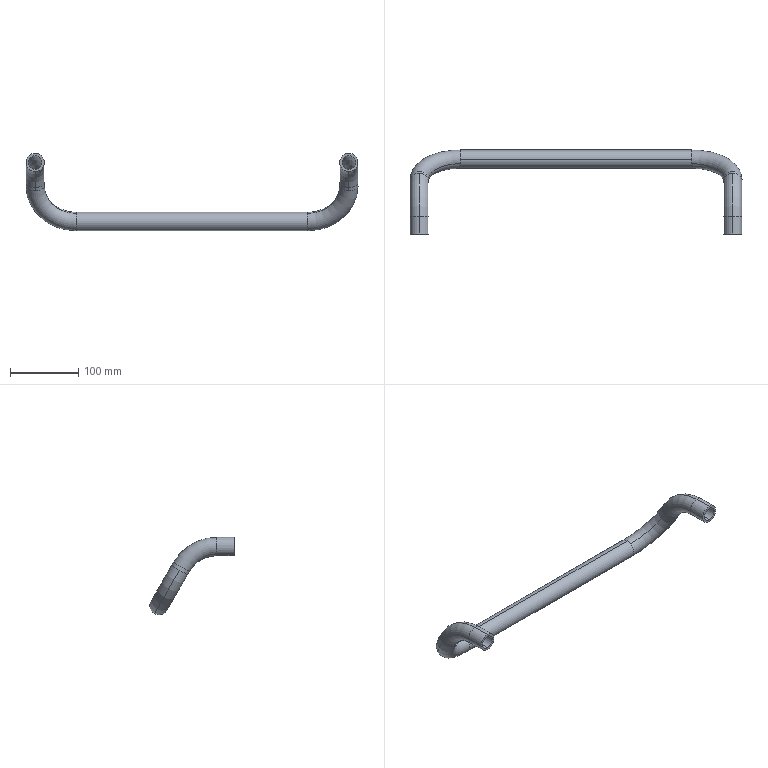Part | STEP file | X77-09101 | 1 solid | 38 faces | box 487 x 123.546 x 113.683 mm | volume 184955 mm3 | cylinder 20 | torus 16 | plane 2 | commonest cylinder face diameters 20 x10 27 x10
STEP:
#1=CARTESIAN_POINT('',(460.,25.359,10.));
#2=VERTEX_POINT('',#1);
#3=CARTESIAN_POINT('',(460.,25.359,-10.));
#4=VERTEX_POINT('',#3);
#5=CARTESIAN_POINT('',(460.,25.359,0.));
#6=DIRECTION('',(0.,1.,0.));
#7=DIRECTION('',(0.,0.,1.));
#8=AXIS2_PLACEMENT_3D('',#5,#6,#7);
#9=CIRCLE('',#8,10.);
#10=EDGE_CURVE('',#2,#4,#9,.T.);
#11=ORIENTED_EDGE('',*,*,#10,.F.);
#12=CARTESIAN_POINT('',(460.,85.981,-25.));
#13=VERTEX_POINT('',#12);
#14=CARTESIAN_POINT('',(460.,25.359,-60.));
#15=DIRECTION('',(-1.,0.,0.));
#16=DIRECTION('',(0.,0.,1.));
#17=AXIS2_PLACEMENT_3D('',#14,#15,#16);
#18=CIRCLE('',#17,70.);
#19=EDGE_CURVE('',#2,#13,#18,.T.);
#20=ORIENTED_EDGE('',*,*,#19,.T.);
#21=CARTESIAN_POINT('',(460.,68.66,-35.));
#22=VERTEX_POINT('',#21);
#23=CARTESIAN_POINT('',(460.,77.321,-30.));
#24=DIRECTION('',(0.,0.5,-0.866));
#25=DIRECTION('',(0.,0.866,0.5));
#26=AXIS2_PLACEMENT_3D('',#23,#24,#25);
#27=CIRCLE('',#26,10.);
#28=EDGE_CURVE('',#13,#22,#27,.T.);
#29=ORIENTED_EDGE('',*,*,#28,.T.);
#30=CARTESIAN_POINT('',(460.,25.359,-60.));
#31=DIRECTION('',(-1.,0.,0.));
#32=DIRECTION('',(0.,0.,1.));
#33=AXIS2_PLACEMENT_3D('',#30,#31,#32);
#34=CIRCLE('',#33,50.);
#35=EDGE_CURVE('',#4,#22,#34,.T.);
#36=ORIENTED_EDGE('',*,*,#35,.F.);
#37=EDGE_LOOP('',(#11,#20,#29,#36));
#38=FACE_OUTER_BOUND('',#37,.T.);
#39=CARTESIAN_POINT('',(460.,25.359,-60.));
#40=DIRECTION('',(-1.,0.,0.));
#41=DIRECTION('',(0.,0.,1.));
#42=AXIS2_PLACEMENT_3D('',#39,#40,#41);
#43=TOROIDAL_SURFACE('',#42,60.,10.);
#44=ADVANCED_FACE('',(#38),#43,.F.);
#45=CARTESIAN_POINT('',(460.,25.359,-13.5));
#46=VERTEX_POINT('',#45);
#47=CARTESIAN_POINT('',(460.,25.359,13.5));
#48=VERTEX_POINT('',#47);
#49=CARTESIAN_POINT('',(460.,25.359,0.));
#50=DIRECTION('',(0.,1.,0.));
#51=DIRECTION('',(0.,0.,1.));
#52=AXIS2_PLACEMENT_3D('',#49,#50,#51);
#53=CIRCLE('',#52,13.5);
#54=EDGE_CURVE('',#46,#48,#53,.T.);
#55=ORIENTED_EDGE('',*,*,#54,.T.);
#56=CARTESIAN_POINT('',(460.,89.012,-23.25));
#57=VERTEX_POINT('',#56);
#58=CARTESIAN_POINT('',(460.,25.359,-60.));
#59=DIRECTION('',(-1.,0.,0.));
#60=DIRECTION('',(0.,0.,1.));
#61=AXIS2_PLACEMENT_3D('',#58,#59,#60);
#62=CIRCLE('',#61,73.5);
#63=EDGE_CURVE('',#48,#57,#62,.T.);
#64=ORIENTED_EDGE('',*,*,#63,.T.);
#65=CARTESIAN_POINT('',(460.,65.629,-36.75));
#66=VERTEX_POINT('',#65);
#67=CARTESIAN_POINT('',(460.,77.321,-30.));
#68=DIRECTION('',(0.,0.5,-0.866));
#69=DIRECTION('',(0.,0.866,0.5));
#70=AXIS2_PLACEMENT_3D('',#67,#68,#69);
#71=CIRCLE('',#70,13.5);
#72=EDGE_CURVE('',#66,#57,#71,.T.);
#73=ORIENTED_EDGE('',*,*,#72,.F.);
#74=CARTESIAN_POINT('',(460.,25.359,-60.));
#75=DIRECTION('',(-1.,0.,0.));
#76=DIRECTION('',(0.,0.,1.));
#77=AXIS2_PLACEMENT_3D('',#74,#75,#76);
#78=CIRCLE('',#77,46.5);
#79=EDGE_CURVE('',#46,#66,#78,.T.);
#80=ORIENTED_EDGE('',*,*,#79,.F.);
#81=EDGE_LOOP('',(#55,#64,#73,#80));
#82=FACE_OUTER_BOUND('',#81,.T.);
#83=CARTESIAN_POINT('',(460.,25.359,-60.));
#84=DIRECTION('',(-1.,0.,0.));
#85=DIRECTION('',(0.,0.,1.));
#86=AXIS2_PLACEMENT_3D('',#83,#84,#85);
#87=TOROIDAL_SURFACE('',#86,60.,13.5);
#88=ADVANCED_FACE('',(#82),#87,.T.);
#89=CARTESIAN_POINT('',(470.,80.046,-34.721));
#90=VERTEX_POINT('',#89);
#91=CARTESIAN_POINT('',(460.,71.386,-39.721));
#92=VERTEX_POINT('',#91);
#93=CARTESIAN_POINT('',(460.,80.046,-34.721));
#94=DIRECTION('',(0.,0.5,-0.866));
#95=DIRECTION('',(0.,0.866,0.5));
#96=AXIS2_PLACEMENT_3D('',#93,#94,#95);
#97=CIRCLE('',#96,10.);
#98=EDGE_CURVE('',#90,#92,#97,.T.);
#99=ORIENTED_EDGE('',*,*,#98,.F.);
#100=CARTESIAN_POINT('',(400.,115.046,-95.343));
#101=VERTEX_POINT('',#100);
#102=CARTESIAN_POINT('',(400.,80.046,-34.721));
#103=DIRECTION('',(0.,0.866,0.5));
#104=DIRECTION('',(0.,-0.5,0.866));
#105=AXIS2_PLACEMENT_3D('',#102,#103,#104);
#106=CIRCLE('',#105,70.);
#107=EDGE_CURVE('',#90,#101,#106,.T.);
#108=ORIENTED_EDGE('',*,*,#107,.T.);
#109=CARTESIAN_POINT('',(400.,110.046,-96.683));
#110=VERTEX_POINT('',#109);
#111=CARTESIAN_POINT('',(400.,110.046,-86.683));
#112=DIRECTION('',(-1.,0.,0.));
#113=DIRECTION('',(0.,0.866,0.5));
#114=AXIS2_PLACEMENT_3D('',#111,#112,#113);
#115=CIRCLE('',#114,10.);
#116=EDGE_CURVE('',#101,#110,#115,.T.);
#117=ORIENTED_EDGE('',*,*,#116,.T.);
#118=CARTESIAN_POINT('',(400.,105.046,-78.023));
#119=VERTEX_POINT('',#118);
#120=CARTESIAN_POINT('',(400.,110.046,-86.683));
#121=DIRECTION('',(-1.,0.,0.));
#122=DIRECTION('',(0.,0.866,0.5));
#123=AXIS2_PLACEMENT_3D('',#120,#121,#122);
#124=CIRCLE('',#123,10.);
#125=EDGE_CURVE('',#110,#119,#124,.T.);
#126=ORIENTED_EDGE('',*,*,#125,.T.);
#127=CARTESIAN_POINT('',(450.,80.046,-34.721));
#128=VERTEX_POINT('',#127);
#129=CARTESIAN_POINT('',(400.,80.046,-34.721));
#130=DIRECTION('',(0.,0.866,0.5));
#131=DIRECTION('',(0.,-0.5,0.866));
#132=AXIS2_PLACEMENT_3D('',#129,#130,#131);
#133=CIRCLE('',#132,50.);
#134=EDGE_CURVE('',#128,#119,#133,.T.);
#135=ORIENTED_EDGE('',*,*,#134,.F.);
#136=CARTESIAN_POINT('',(460.,80.046,-34.721));
#137=DIRECTION('',(0.,0.5,-0.866));
#138=DIRECTION('',(0.,0.866,0.5));
#139=AXIS2_PLACEMENT_3D('',#136,#137,#138);
#140=CIRCLE('',#139,10.);
#141=EDGE_CURVE('',#92,#128,#140,.T.);
#142=ORIENTED_EDGE('',*,*,#141,.F.);
#143=EDGE_LOOP('',(#99,#108,#117,#126,#135,#142));
#144=FACE_OUTER_BOUND('',#143,.T.);
#145=CARTESIAN_POINT('',(400.,80.046,-34.721));
#146=DIRECTION('',(0.,0.866,0.5));
#147=DIRECTION('',(0.,-0.5,0.866));
#148=AXIS2_PLACEMENT_3D('',#145,#146,#147);
#149=TOROIDAL_SURFACE('',#148,60.,10.);
#150=ADVANCED_FACE('',(#144),#149,.F.);
#151=CARTESIAN_POINT('',(460.,91.738,-27.971));
#152=VERTEX_POINT('',#151);
#153=CARTESIAN_POINT('',(473.5,80.046,-34.721));
#154=VERTEX_POINT('',#153);
#155=CARTESIAN_POINT('',(460.,80.046,-34.721));
#156=DIRECTION('',(0.,0.5,-0.866));
#157=DIRECTION('',(0.,0.866,0.5));
#158=AXIS2_PLACEMENT_3D('',#155,#156,#157);
#159=CIRCLE('',#158,13.5);
#160=EDGE_CURVE('',#152,#154,#159,.T.);
#161=ORIENTED_EDGE('',*,*,#160,.T.);
#162=CARTESIAN_POINT('',(400.,116.796,-98.374));
#163=VERTEX_POINT('',#162);
#164=CARTESIAN_POINT('',(400.,80.046,-34.721));
#165=DIRECTION('',(0.,0.866,0.5));
#166=DIRECTION('',(0.,-0.5,0.866));
#167=AXIS2_PLACEMENT_3D('',#164,#165,#166);
#168=CIRCLE('',#167,73.5);
#169=EDGE_CURVE('',#154,#163,#168,.T.);
#170=ORIENTED_EDGE('',*,*,#169,.T.);
#171=CARTESIAN_POINT('',(400.,110.046,-73.183));
#172=VERTEX_POINT('',#171);
#173=CARTESIAN_POINT('',(400.,110.046,-86.683));
#174=DIRECTION('',(-1.,0.,0.));
#175=DIRECTION('',(0.,0.866,0.5));
#176=AXIS2_PLACEMENT_3D('',#173,#174,#175);
#177=CIRCLE('',#176,13.5);
#178=EDGE_CURVE('',#172,#163,#177,.T.);
#179=ORIENTED_EDGE('',*,*,#178,.F.);
#180=CARTESIAN_POINT('',(400.,103.296,-74.992));
#181=VERTEX_POINT('',#180);
#182=CARTESIAN_POINT('',(400.,110.046,-86.683));
#183=DIRECTION('',(-1.,0.,0.));
#184=DIRECTION('',(0.,0.866,0.5));
#185=AXIS2_PLACEMENT_3D('',#182,#183,#184);
#186=CIRCLE('',#185,13.5);
#187=EDGE_CURVE('',#181,#172,#186,.T.);
#188=ORIENTED_EDGE('',*,*,#187,.F.);
#189=CARTESIAN_POINT('',(446.5,80.046,-34.721));
#190=VERTEX_POINT('',#189);
#191=CARTESIAN_POINT('',(400.,80.046,-34.721));
#192=DIRECTION('',(0.,0.866,0.5));
#193=DIRECTION('',(0.,-0.5,0.866));
#194=AXIS2_PLACEMENT_3D('',#191,#192,#193);
#195=CIRCLE('',#194,46.5);
#196=EDGE_CURVE('',#190,#181,#195,.T.);
#197=ORIENTED_EDGE('',*,*,#196,.F.);
#198=CARTESIAN_POINT('',(460.,80.046,-34.721));
#199=DIRECTION('',(0.,0.5,-0.866));
#200=DIRECTION('',(0.,0.866,0.5));
#201=AXIS2_PLACEMENT_3D('',#198,#199,#200);
#202=CIRCLE('',#201,13.5);
#203=EDGE_CURVE('',#190,#152,#202,.T.);
#204=ORIENTED_EDGE('',*,*,#203,.T.);
#205=EDGE_LOOP('',(#161,#170,#179,#188,#197,#204));
#206=FACE_OUTER_BOUND('',#205,.T.);
#207=CARTESIAN_POINT('',(400.,80.046,-34.721));
#208=DIRECTION('',(0.,0.866,0.5));
#209=DIRECTION('',(0.,-0.5,0.866));
#210=AXIS2_PLACEMENT_3D('',#207,#208,#209);
#211=TOROIDAL_SURFACE('',#210,60.,13.5);
#212=ADVANCED_FACE('',(#206),#211,.T.);
#213=CARTESIAN_POINT('',(60.,115.046,-95.343));
#214=VERTEX_POINT('',#213);
#215=CARTESIAN_POINT('',(60.,110.046,-96.683));
#216=VERTEX_POINT('',#215);
#217=CARTESIAN_POINT('',(60.,110.046,-86.683));
#218=DIRECTION('',(-1.,0.,0.));
#219=DIRECTION('',(0.,0.866,0.5));
#220=AXIS2_PLACEMENT_3D('',#217,#218,#219);
#221=CIRCLE('',#220,10.);
#222=EDGE_CURVE('',#214,#216,#221,.T.);
#223=ORIENTED_EDGE('',*,*,#222,.F.);
#224=CARTESIAN_POINT('',(-10.,80.046,-34.721));
#225=VERTEX_POINT('',#224);
#226=CARTESIAN_POINT('',(60.,80.046,-34.721));
#227=DIRECTION('',(0.,0.866,0.5));
#228=DIRECTION('',(0.,-0.5,0.866));
#229=AXIS2_PLACEMENT_3D('',#226,#227,#228);
#230=CIRCLE('',#229,70.);
#231=EDGE_CURVE('',#214,#225,#230,.T.);
#232=ORIENTED_EDGE('',*,*,#231,.T.);
#233=CARTESIAN_POINT('',(0.,71.386,-39.721));
#234=VERTEX_POINT('',#233);
#235=CARTESIAN_POINT('',(0.,80.046,-34.721));
#236=DIRECTION('',(0.,-0.5,0.866));
#237=DIRECTION('',(0.,0.866,0.5));
#238=AXIS2_PLACEMENT_3D('',#235,#236,#237);
#239=CIRCLE('',#238,10.);
#240=EDGE_CURVE('',#225,#234,#239,.T.);
#241=ORIENTED_EDGE('',*,*,#240,.T.);
#242=CARTESIAN_POINT('',(10.,80.046,-34.721));
#243=VERTEX_POINT('',#242);
#244=CARTESIAN_POINT('',(0.,80.046,-34.721));
#245=DIRECTION('',(0.,-0.5,0.866));
#246=DIRECTION('',(0.,0.866,0.5));
#247=AXIS2_PLACEMENT_3D('',#244,#245,#246);
#248=CIRCLE('',#247,10.);
#249=EDGE_CURVE('',#234,#243,#248,.T.);
#250=ORIENTED_EDGE('',*,*,#249,.T.);
#251=CARTESIAN_POINT('',(60.,105.046,-78.023));
#252=VERTEX_POINT('',#251);
#253=CARTESIAN_POINT('',(60.,80.046,-34.721));
#254=DIRECTION('',(0.,0.866,0.5));
#255=DIRECTION('',(0.,-0.5,0.866));
#256=AXIS2_PLACEMENT_3D('',#253,#254,#255);
#257=CIRCLE('',#256,50.);
#258=EDGE_CURVE('',#252,#243,#257,.T.);
#259=ORIENTED_EDGE('',*,*,#258,.F.);
#260=CARTESIAN_POINT('',(60.,110.046,-86.683));
#261=DIRECTION('',(-1.,0.,0.));
#262=DIRECTION('',(0.,0.866,0.5));
#263=AXIS2_PLACEMENT_3D('',#260,#261,#262);
#264=CIRCLE('',#263,10.);
#265=EDGE_CURVE('',#216,#252,#264,.T.);
#266=ORIENTED_EDGE('',*,*,#265,.F.);
#267=EDGE_LOOP('',(#223,#232,#241,#250,#259,#266));
#268=FACE_OUTER_BOUND('',#267,.T.);
#269=CARTESIAN_POINT('',(60.,80.046,-34.721));
#270=DIRECTION('',(0.,0.866,0.5));
#271=DIRECTION('',(0.,-0.5,0.866));
#272=AXIS2_PLACEMENT_3D('',#269,#270,#271);
#273=TOROIDAL_SURFACE('',#272,60.,10.);
#274=ADVANCED_FACE('',(#268),#273,.F.);
#275=CARTESIAN_POINT('',(60.,110.046,-73.183));
#276=VERTEX_POINT('',#275);
#277=CARTESIAN_POINT('',(60.,116.796,-98.374));
#278=VERTEX_POINT('',#277);
#279=CARTESIAN_POINT('',(60.,110.046,-86.683));
#280=DIRECTION('',(-1.,0.,0.));
#281=DIRECTION('',(0.,0.866,0.5));
#282=AXIS2_PLACEMENT_3D('',#279,#280,#281);
#283=CIRCLE('',#282,13.5);
#284=EDGE_CURVE('',#276,#278,#283,.T.);
#285=ORIENTED_EDGE('',*,*,#284,.T.);
#286=CARTESIAN_POINT('',(-13.5,80.046,-34.721));
#287=VERTEX_POINT('',#286);
#288=CARTESIAN_POINT('',(60.,80.046,-34.721));
#289=DIRECTION('',(0.,0.866,0.5));
#290=DIRECTION('',(0.,-0.5,0.866));
#291=AXIS2_PLACEMENT_3D('',#288,#289,#290);
#292=CIRCLE('',#291,73.5);
#293=EDGE_CURVE('',#278,#287,#292,.T.);
#294=ORIENTED_EDGE('',*,*,#293,.T.);
#295=CARTESIAN_POINT('',(0.,91.738,-27.971));
#296=VERTEX_POINT('',#295);
#297=CARTESIAN_POINT('',(0.,80.046,-34.721));
#298=DIRECTION('',(0.,-0.5,0.866));
#299=DIRECTION('',(0.,0.866,0.5));
#300=AXIS2_PLACEMENT_3D('',#297,#298,#299);
#301=CIRCLE('',#300,13.5);
#302=EDGE_CURVE('',#296,#287,#301,.T.);
#303=ORIENTED_EDGE('',*,*,#302,.F.);
#304=CARTESIAN_POINT('',(13.5,80.046,-34.721));
#305=VERTEX_POINT('',#304);
#306=CARTESIAN_POINT('',(0.,80.046,-34.721));
#307=DIRECTION('',(0.,-0.5,0.866));
#308=DIRECTION('',(0.,0.866,0.5));
#309=AXIS2_PLACEMENT_3D('',#306,#307,#308);
#310=CIRCLE('',#309,13.5);
#311=EDGE_CURVE('',#305,#296,#310,.T.);
#312=ORIENTED_EDGE('',*,*,#311,.F.);
#313=CARTESIAN_POINT('',(60.,103.296,-74.992));
#314=VERTEX_POINT('',#313);
#315=CARTESIAN_POINT('',(60.,80.046,-34.721));
#316=DIRECTION('',(0.,0.866,0.5));
#317=DIRECTION('',(0.,-0.5,0.866));
#318=AXIS2_PLACEMENT_3D('',#315,#316,#317);
#319=CIRCLE('',#318,46.5);
#320=EDGE_CURVE('',#314,#305,#319,.T.);
#321=ORIENTED_EDGE('',*,*,#320,.F.);
#322=CARTESIAN_POINT('',(60.,110.046,-86.683));
#323=DIRECTION('',(-1.,0.,0.));
#324=DIRECTION('',(0.,0.866,0.5));
#325=AXIS2_PLACEMENT_3D('',#322,#323,#324);
#326=CIRCLE('',#325,13.5);
#327=EDGE_CURVE('',#314,#276,#326,.T.);
#328=ORIENTED_EDGE('',*,*,#327,.T.);
#329=EDGE_LOOP('',(#285,#294,#303,#312,#321,#328));
#330=FACE_OUTER_BOUND('',#329,.T.);
#331=CARTESIAN_POINT('',(60.,80.046,-34.721));
#332=DIRECTION('',(0.,0.866,0.5));
#333=DIRECTION('',(0.,-0.5,0.866));
#334=AXIS2_PLACEMENT_3D('',#331,#332,#333);
#335=TOROIDAL_SURFACE('',#334,60.,13.5);
#336=ADVANCED_FACE('',(#330),#335,.T.);
#337=CARTESIAN_POINT('',(0.,25.359,10.));
#338=VERTEX_POINT('',#337);
#339=CARTESIAN_POINT('',(0.,25.359,-10.));
#340=VERTEX_POINT('',#339);
#341=CARTESIAN_POINT('',(0.,25.359,0.));
#342=DIRECTION('',(0.,1.,0.));
#343=DIRECTION('',(0.,0.,1.));
#344=AXIS2_PLACEMENT_3D('',#341,#342,#343);
#345=CIRCLE('',#344,10.);
#346=EDGE_CURVE('',#338,#340,#345,.T.);
#347=ORIENTED_EDGE('',*,*,#346,.F.);
#348=CARTESIAN_POINT('',(0.,85.981,-25.));
#349=VERTEX_POINT('',#348);
#350=CARTESIAN_POINT('',(0.,25.359,-60.));
#351=DIRECTION('',(-1.,0.,0.));
#352=DIRECTION('',(0.,0.,1.));
#353=AXIS2_PLACEMENT_3D('',#350,#351,#352);
#354=CIRCLE('',#353,70.);
#355=EDGE_CURVE('',#338,#349,#354,.T.);
#356=ORIENTED_EDGE('',*,*,#355,.T.);
#357=CARTESIAN_POINT('',(0.,68.66,-35.));
#358=VERTEX_POINT('',#357);
#359=CARTESIAN_POINT('',(0.,77.321,-30.));
#360=DIRECTION('',(0.,0.5,-0.866));
#361=DIRECTION('',(0.,0.866,0.5));
#362=AXIS2_PLACEMENT_3D('',#359,#360,#361);
#363=CIRCLE('',#362,10.);
#364=EDGE_CURVE('',#349,#358,#363,.T.);
#365=ORIENTED_EDGE('',*,*,#364,.T.);
#366=CARTESIAN_POINT('',(0.,25.359,-60.));
#367=DIRECTION('',(-1.,0.,0.));
#368=DIRECTION('',(0.,0.,1.));
#369=AXIS2_PLACEMENT_3D('',#366,#367,#368);
#370=CIRCLE('',#369,50.);
#371=EDGE_CURVE('',#340,#358,#370,.T.);
#372=ORIENTED_EDGE('',*,*,#371,.F.);
#373=EDGE_LOOP('',(#347,#356,#365,#372));
#374=FACE_OUTER_BOUND('',#373,.T.);
#375=CARTESIAN_POINT('',(0.,25.359,-60.));
#376=DIRECTION('',(-1.,0.,0.));
#377=DIRECTION('',(0.,0.,1.));
#378=AXIS2_PLACEMENT_3D('',#375,#376,#377);
#379=TOROIDAL_SURFACE('',#378,60.,10.);
#380=ADVANCED_FACE('',(#374),#379,.F.);
#381=CARTESIAN_POINT('',(0.,25.359,-13.5));
#382=VERTEX_POINT('',#381);
#383=CARTESIAN_POINT('',(0.,25.359,13.5));
#384=VERTEX_POINT('',#383);
#385=CARTESIAN_POINT('',(0.,25.359,0.));
#386=DIRECTION('',(0.,1.,0.));
#387=DIRECTION('',(0.,0.,1.));
#388=AXIS2_PLACEMENT_3D('',#385,#386,#387);
#389=CIRCLE('',#388,13.5);
#390=EDGE_CURVE('',#382,#384,#389,.T.);
#391=ORIENTED_EDGE('',*,*,#390,.T.);
#392=CARTESIAN_POINT('',(0.,89.012,-23.25));
#393=VERTEX_POINT('',#392);
#394=CARTESIAN_POINT('',(0.,25.359,-60.));
#395=DIRECTION('',(-1.,0.,0.));
#396=DIRECTION('',(0.,0.,1.));
#397=AXIS2_PLACEMENT_3D('',#394,#395,#396);
#398=CIRCLE('',#397,73.5);
#399=EDGE_CURVE('',#384,#393,#398,.T.);
#400=ORIENTED_EDGE('',*,*,#399,.T.);
#401=CARTESIAN_POINT('',(0.,65.629,-36.75));
#402=VERTEX_POINT('',#401);
#403=CARTESIAN_POINT('',(0.,77.321,-30.));
#404=DIRECTION('',(0.,0.5,-0.866));
#405=DIRECTION('',(0.,0.866,0.5));
#406=AXIS2_PLACEMENT_3D('',#403,#404,#405);
#407=CIRCLE('',#406,13.5);
#408=EDGE_CURVE('',#402,#393,#407,.T.);
#409=ORIENTED_EDGE('',*,*,#408,.F.);
#410=CARTESIAN_POINT('',(0.,25.359,-60.));
#411=DIRECTION('',(-1.,0.,0.));
#412=DIRECTION('',(0.,0.,1.));
#413=AXIS2_PLACEMENT_3D('',#410,#411,#412);
#414=CIRCLE('',#413,46.5);
#415=EDGE_CURVE('',#382,#402,#414,.T.);
#416=ORIENTED_EDGE('',*,*,#415,.F.);
#417=EDGE_LOOP('',(#391,#400,#409,#416));
#418=FACE_OUTER_BOUND('',#417,.T.);
#419=CARTESIAN_POINT('',(0.,25.359,-60.));
#420=DIRECTION('',(-1.,0.,0.));
#421=DIRECTION('',(0.,0.,1.));
#422=AXIS2_PLACEMENT_3D('',#419,#420,#421);
#423=TOROIDAL_SURFACE('',#422,60.,13.5);
#424=ADVANCED_FACE('',(#418),#423,.T.);
#425=CARTESIAN_POINT('',(460.,25.359,0.));
#426=DIRECTION('',(0.,1.,0.));
#427=DIRECTION('',(0.,0.,1.));
#428=AXIS2_PLACEMENT_3D('',#425,#426,#427);
#429=CIRCLE('',#428,13.5);
#430=EDGE_CURVE('',#48,#46,#429,.T.);
#431=ORIENTED_EDGE('',*,*,#430,.F.);
#432=CARTESIAN_POINT('',(460.,0.,13.5));
#433=VERTEX_POINT('',#432);
#434=CARTESIAN_POINT('',(460.,25.359,13.5));
#435=DIRECTION('',(0.,-1.,0.));
#436=VECTOR('',#435,1000.);
#437=LINE('',#434,#436);
#438=EDGE_CURVE('',#48,#433,#437,.T.);
#439=ORIENTED_EDGE('',*,*,#438,.T.);
#440=CARTESIAN_POINT('',(460.,0.,-13.5));
#441=VERTEX_POINT('',#440);
#442=CARTESIAN_POINT('',(460.,0.,0.));
#443=DIRECTION('',(0.,1.,0.));
#444=DIRECTION('',(0.,0.,1.));
#445=AXIS2_PLACEMENT_3D('',#442,#443,#444);
#446=CIRCLE('',#445,13.5);
#447=EDGE_CURVE('',#433,#441,#446,.T.);
#448=ORIENTED_EDGE('',*,*,#447,.T.);
#449=CARTESIAN_POINT('',(460.,25.359,-13.5));
#450=DIRECTION('',(0.,-1.,0.));
#451=VECTOR('',#450,1000.);
#452=LINE('',#449,#451);
#453=EDGE_CURVE('',#46,#441,#452,.T.);
#454=ORIENTED_EDGE('',*,*,#453,.F.);
#455=EDGE_LOOP('',(#431,#439,#448,#454));
#456=FACE_OUTER_BOUND('',#455,.T.);
#457=CARTESIAN_POINT('',(460.,25.359,0.));
#458=DIRECTION('',(0.,-1.,0.));
#459=DIRECTION('',(0.,0.,-1.));
#460=AXIS2_PLACEMENT_3D('',#457,#458,#459);
#461=CYLINDRICAL_SURFACE('',#460,13.5);
#462=ADVANCED_FACE('',(#456),#461,.T.);
#463=CARTESIAN_POINT('',(460.,25.359,0.));
#464=DIRECTION('',(0.,1.,0.));
#465=DIRECTION('',(0.,0.,1.));
#466=AXIS2_PLACEMENT_3D('',#463,#464,#465);
#467=CIRCLE('',#466,10.);
#468=EDGE_CURVE('',#4,#2,#467,.T.);
#469=ORIENTED_EDGE('',*,*,#468,.T.);
#470=CARTESIAN_POINT('',(460.,0.,10.));
#471=VERTEX_POINT('',#470);
#472=CARTESIAN_POINT('',(460.,25.359,10.));
#473=DIRECTION('',(0.,-1.,0.));
#474=VECTOR('',#473,1000.);
#475=LINE('',#472,#474);
#476=EDGE_CURVE('',#2,#471,#475,.T.);
#477=ORIENTED_EDGE('',*,*,#476,.T.);
#478=CARTESIAN_POINT('',(460.,0.,-10.));
#479=VERTEX_POINT('',#478);
#480=CARTESIAN_POINT('',(460.,0.,0.));
#481=DIRECTION('',(0.,1.,0.));
#482=DIRECTION('',(0.,0.,1.));
#483=AXIS2_PLACEMENT_3D('',#480,#481,#482);
#484=CIRCLE('',#483,10.);
#485=EDGE_CURVE('',#479,#471,#484,.T.);
#486=ORIENTED_EDGE('',*,*,#485,.F.);
#487=CARTESIAN_POINT('',(460.,25.359,-10.));
#488=DIRECTION('',(0.,-1.,0.));
#489=VECTOR('',#488,1000.);
#490=LINE('',#487,#489);
#491=EDGE_CURVE('',#4,#479,#490,.T.);
#492=ORIENTED_EDGE('',*,*,#491,.F.);
#493=EDGE_LOOP('',(#469,#477,#486,#492));
#494=FACE_OUTER_BOUND('',#493,.T.);
#495=CARTESIAN_POINT('',(460.,25.359,0.));
#496=DIRECTION('',(0.,-1.,0.));
#497=DIRECTION('',(0.,0.,-1.));
#498=AXIS2_PLACEMENT_3D('',#495,#496,#497);
#499=CYLINDRICAL_SURFACE('',#498,10.);
#500=ADVANCED_FACE('',(#494),#499,.F.);
#501=ORIENTED_EDGE('',*,*,#160,.F.);
#502=CARTESIAN_POINT('',(460.,91.738,-27.971));
#503=DIRECTION('',(0.,-0.5,0.866));
#504=VECTOR('',#503,1000.);
#505=LINE('',#502,#504);
#506=EDGE_CURVE('',#152,#57,#505,.T.);
#507=ORIENTED_EDGE('',*,*,#506,.T.);
#508=CARTESIAN_POINT('',(460.,77.321,-30.));
#509=DIRECTION('',(0.,0.5,-0.866));
#510=DIRECTION('',(0.,0.866,0.5));
#511=AXIS2_PLACEMENT_3D('',#508,#509,#510);
#512=CIRCLE('',#511,13.5);
#513=EDGE_CURVE('',#57,#66,#512,.T.);
#514=ORIENTED_EDGE('',*,*,#513,.T.);
#515=CARTESIAN_POINT('',(460.,68.355,-41.471));
#516=VERTEX_POINT('',#515);
#517=CARTESIAN_POINT('',(460.,68.355,-41.471));
#518=DIRECTION('',(0.,-0.5,0.866));
#519=VECTOR('',#518,1000.);
#520=LINE('',#517,#519);
#521=EDGE_CURVE('',#516,#66,#520,.T.);
#522=ORIENTED_EDGE('',*,*,#521,.F.);
#523=CARTESIAN_POINT('',(460.,80.046,-34.721));
#524=DIRECTION('',(0.,0.5,-0.866));
#525=DIRECTION('',(0.,0.866,0.5));
#526=AXIS2_PLACEMENT_3D('',#523,#524,#525);
#527=CIRCLE('',#526,13.5);
#528=EDGE_CURVE('',#154,#516,#527,.T.);
#529=ORIENTED_EDGE('',*,*,#528,.F.);
#530=EDGE_LOOP('',(#501,#507,#514,#522,#529));
#531=FACE_OUTER_BOUND('',#530,.T.);
#532=CARTESIAN_POINT('',(460.,80.046,-34.721));
#533=DIRECTION('',(0.,-0.5,0.866));
#534=DIRECTION('',(0.,-0.866,-0.5));
#535=AXIS2_PLACEMENT_3D('',#532,#533,#534);
#536=CYLINDRICAL_SURFACE('',#535,13.5);
#537=ADVANCED_FACE('',(#531),#536,.T.);
#538=ORIENTED_EDGE('',*,*,#141,.T.);
#539=CARTESIAN_POINT('',(460.,88.707,-29.721));
#540=VERTEX_POINT('',#539);
#541=CARTESIAN_POINT('',(460.,80.046,-34.721));
#542=DIRECTION('',(0.,0.5,-0.866));
#543=DIRECTION('',(0.,0.866,0.5));
#544=AXIS2_PLACEMENT_3D('',#541,#542,#543);
#545=CIRCLE('',#544,10.);
#546=EDGE_CURVE('',#128,#540,#545,.T.);
#547=ORIENTED_EDGE('',*,*,#546,.T.);
#548=CARTESIAN_POINT('',(460.,88.707,-29.721));
#549=DIRECTION('',(0.,-0.5,0.866));
#550=VECTOR('',#549,1000.);
#551=LINE('',#548,#550);
#552=EDGE_CURVE('',#540,#13,#551,.T.);
#553=ORIENTED_EDGE('',*,*,#552,.T.);
#554=CARTESIAN_POINT('',(460.,77.321,-30.));
#555=DIRECTION('',(0.,0.5,-0.866));
#556=DIRECTION('',(0.,0.866,0.5));
#557=AXIS2_PLACEMENT_3D('',#554,#555,#556);
#558=CIRCLE('',#557,10.);
#559=EDGE_CURVE('',#22,#13,#558,.T.);
#560=ORIENTED_EDGE('',*,*,#559,.F.);
#561=CARTESIAN_POINT('',(460.,71.386,-39.721));
#562=DIRECTION('',(0.,-0.5,0.866));
#563=VECTOR('',#562,1000.);
#564=LINE('',#561,#563);
#565=EDGE_CURVE('',#92,#22,#564,.T.);
#566=ORIENTED_EDGE('',*,*,#565,.F.);
#567=EDGE_LOOP('',(#538,#547,#553,#560,#566));
#568=FACE_OUTER_BOUND('',#567,.T.);
#569=CARTESIAN_POINT('',(460.,80.046,-34.721));
#570=DIRECTION('',(0.,-0.5,0.866));
#571=DIRECTION('',(0.,-0.866,-0.5));
#572=AXIS2_PLACEMENT_3D('',#569,#570,#571);
#573=CYLINDRICAL_SURFACE('',#572,10.);
#574=ADVANCED_FACE('',(#568),#573,.F.);
#575=ORIENTED_EDGE('',*,*,#125,.F.);
#576=CARTESIAN_POINT('',(400.,110.046,-96.683));
#577=DIRECTION('',(-1.,0.,0.));
#578=VECTOR('',#577,1000.);
#579=LINE('',#576,#578);
#580=EDGE_CURVE('',#110,#216,#579,.T.);
#581=ORIENTED_EDGE('',*,*,#580,.T.);
#582=ORIENTED_EDGE('',*,*,#265,.T.);
#583=CARTESIAN_POINT('',(60.,110.046,-76.683));
#584=VERTEX_POINT('',#583);
#585=CARTESIAN_POINT('',(60.,110.046,-86.683));
#586=DIRECTION('',(-1.,0.,0.));
#587=DIRECTION('',(0.,0.866,0.5));
#588=AXIS2_PLACEMENT_3D('',#585,#586,#587);
#589=CIRCLE('',#588,10.);
#590=EDGE_CURVE('',#252,#584,#589,.T.);
#591=ORIENTED_EDGE('',*,*,#590,.T.);
#592=CARTESIAN_POINT('',(400.,110.046,-76.683));
#593=VERTEX_POINT('',#592);
#594=CARTESIAN_POINT('',(400.,110.046,-76.683));
#595=DIRECTION('',(-1.,0.,0.));
#596=VECTOR('',#595,1000.);
#597=LINE('',#594,#596);
#598=EDGE_CURVE('',#593,#584,#597,.T.);
#599=ORIENTED_EDGE('',*,*,#598,.F.);
#600=CARTESIAN_POINT('',(400.,110.046,-86.683));
#601=DIRECTION('',(-1.,0.,0.));
#602=DIRECTION('',(0.,0.866,0.5));
#603=AXIS2_PLACEMENT_3D('',#600,#601,#602);
#604=CIRCLE('',#603,10.);
#605=EDGE_CURVE('',#119,#593,#604,.T.);
#606=ORIENTED_EDGE('',*,*,#605,.F.);
#607=EDGE_LOOP('',(#575,#581,#582,#591,#599,#606));
#608=FACE_OUTER_BOUND('',#607,.T.);
#609=CARTESIAN_POINT('',(400.,110.046,-86.683));
#610=DIRECTION('',(-1.,0.,0.));
#611=DIRECTION('',(0.,0.,1.));
#612=AXIS2_PLACEMENT_3D('',#609,#610,#611);
#613=CYLINDRICAL_SURFACE('',#612,10.);
#614=ADVANCED_FACE('',(#608),#613,.F.);
#615=ORIENTED_EDGE('',*,*,#178,.T.);
#616=CARTESIAN_POINT('',(400.,110.046,-100.183));
#617=VERTEX_POINT('',#616);
#618=CARTESIAN_POINT('',(400.,110.046,-86.683));
#619=DIRECTION('',(-1.,0.,0.));
#620=DIRECTION('',(0.,0.866,0.5));
#621=AXIS2_PLACEMENT_3D('',#618,#619,#620);
#622=CIRCLE('',#621,13.5);
#623=EDGE_CURVE('',#163,#617,#622,.T.);
#624=ORIENTED_EDGE('',*,*,#623,.T.);
#625=CARTESIAN_POINT('',(60.,110.046,-100.183));
#626=VERTEX_POINT('',#625);
#627=CARTESIAN_POINT('',(400.,110.046,-100.183));
#628=DIRECTION('',(-1.,0.,0.));
#629=VECTOR('',#628,1000.);
#630=LINE('',#627,#629);
#631=EDGE_CURVE('',#617,#626,#630,.T.);
#632=ORIENTED_EDGE('',*,*,#631,.T.);
#633=CARTESIAN_POINT('',(60.,110.046,-86.683));
#634=DIRECTION('',(-1.,0.,0.));
#635=DIRECTION('',(0.,0.866,0.5));
#636=AXIS2_PLACEMENT_3D('',#633,#634,#635);
#637=CIRCLE('',#636,13.5);
#638=EDGE_CURVE('',#278,#626,#637,.T.);
#639=ORIENTED_EDGE('',*,*,#638,.F.);
#640=ORIENTED_EDGE('',*,*,#284,.F.);
#641=CARTESIAN_POINT('',(400.,110.046,-73.183));
#642=DIRECTION('',(-1.,0.,0.));
#643=VECTOR('',#642,1000.);
#644=LINE('',#641,#643);
#645=EDGE_CURVE('',#172,#276,#644,.T.);
#646=ORIENTED_EDGE('',*,*,#645,.F.);
#647=EDGE_LOOP('',(#615,#624,#632,#639,#640,#646));
#648=FACE_OUTER_BOUND('',#647,.T.);
#649=CARTESIAN_POINT('',(400.,110.046,-86.683));
#650=DIRECTION('',(-1.,0.,0.));
#651=DIRECTION('',(0.,0.,1.));
#652=AXIS2_PLACEMENT_3D('',#649,#650,#651);
#653=CYLINDRICAL_SURFACE('',#652,13.5);
#654=ADVANCED_FACE('',(#648),#653,.T.);
#655=CARTESIAN_POINT('',(0.,25.359,0.));
#656=DIRECTION('',(0.,1.,0.));
#657=DIRECTION('',(0.,0.,1.));
#658=AXIS2_PLACEMENT_3D('',#655,#656,#657);
#659=CIRCLE('',#658,13.5);
#660=EDGE_CURVE('',#384,#382,#659,.T.);
#661=ORIENTED_EDGE('',*,*,#660,.F.);
#662=CARTESIAN_POINT('',(0.,0.,13.5));
#663=VERTEX_POINT('',#662);
#664=CARTESIAN_POINT('',(0.,25.359,13.5));
#665=DIRECTION('',(0.,-1.,0.));
#666=VECTOR('',#665,1000.);
#667=LINE('',#664,#666);
#668=EDGE_CURVE('',#384,#663,#667,.T.);
#669=ORIENTED_EDGE('',*,*,#668,.T.);
#670=CARTESIAN_POINT('',(0.,0.,-13.5));
#671=VERTEX_POINT('',#670);
#672=CARTESIAN_POINT('',(0.,0.,0.));
#673=DIRECTION('',(0.,1.,0.));
#674=DIRECTION('',(0.,0.,1.));
#675=AXIS2_PLACEMENT_3D('',#672,#673,#674);
#676=CIRCLE('',#675,13.5);
#677=EDGE_CURVE('',#663,#671,#676,.T.);
#678=ORIENTED_EDGE('',*,*,#677,.T.);
#679=CARTESIAN_POINT('',(0.,25.359,-13.5));
#680=DIRECTION('',(0.,-1.,0.));
#681=VECTOR('',#680,1000.);
#682=LINE('',#679,#681);
#683=EDGE_CURVE('',#382,#671,#682,.T.);
#684=ORIENTED_EDGE('',*,*,#683,.F.);
#685=EDGE_LOOP('',(#661,#669,#678,#684));
#686=FACE_OUTER_BOUND('',#685,.T.);
#687=CARTESIAN_POINT('',(0.,25.359,0.));
#688=DIRECTION('',(0.,-1.,0.));
#689=DIRECTION('',(0.,0.,-1.));
#690=AXIS2_PLACEMENT_3D('',#687,#688,#689);
#691=CYLINDRICAL_SURFACE('',#690,13.5);
#692=ADVANCED_FACE('',(#686),#691,.T.);
#693=CARTESIAN_POINT('',(0.,25.359,0.));
#694=DIRECTION('',(0.,1.,0.));
#695=DIRECTION('',(0.,0.,1.));
#696=AXIS2_PLACEMENT_3D('',#693,#694,#695);
#697=CIRCLE('',#696,10.);
#698=EDGE_CURVE('',#340,#338,#697,.T.);
#699=ORIENTED_EDGE('',*,*,#698,.T.);
#700=CARTESIAN_POINT('',(0.,0.,10.));
#701=VERTEX_POINT('',#700);
#702=CARTESIAN_POINT('',(0.,25.359,10.));
#703=DIRECTION('',(0.,-1.,0.));
#704=VECTOR('',#703,1000.);
#705=LINE('',#702,#704);
#706=EDGE_CURVE('',#338,#701,#705,.T.);
#707=ORIENTED_EDGE('',*,*,#706,.T.);
#708=CARTESIAN_POINT('',(0.,0.,-10.));
#709=VERTEX_POINT('',#708);
#710=CARTESIAN_POINT('',(0.,0.,0.));
#711=DIRECTION('',(0.,1.,0.));
#712=DIRECTION('',(0.,0.,1.));
#713=AXIS2_PLACEMENT_3D('',#710,#711,#712);
#714=CIRCLE('',#713,10.);
#715=EDGE_CURVE('',#709,#701,#714,.T.);
#716=ORIENTED_EDGE('',*,*,#715,.F.);
#717=CARTESIAN_POINT('',(0.,25.359,-10.));
#718=DIRECTION('',(0.,-1.,0.));
#719=VECTOR('',#718,1000.);
#720=LINE('',#717,#719);
#721=EDGE_CURVE('',#340,#709,#720,.T.);
#722=ORIENTED_EDGE('',*,*,#721,.F.);
#723=EDGE_LOOP('',(#699,#707,#716,#722));
#724=FACE_OUTER_BOUND('',#723,.T.);
#725=CARTESIAN_POINT('',(0.,25.359,0.));
#726=DIRECTION('',(0.,-1.,0.));
#727=DIRECTION('',(0.,0.,-1.));
#728=AXIS2_PLACEMENT_3D('',#725,#726,#727);
#729=CYLINDRICAL_SURFACE('',#728,10.);
#730=ADVANCED_FACE('',(#724),#729,.F.);
#731=CARTESIAN_POINT('',(0.,77.321,-30.));
#732=DIRECTION('',(0.,0.5,-0.866));
#733=DIRECTION('',(0.,0.866,0.5));
#734=AXIS2_PLACEMENT_3D('',#731,#732,#733);
#735=CIRCLE('',#734,10.);
#736=EDGE_CURVE('',#358,#349,#735,.T.);
#737=ORIENTED_EDGE('',*,*,#736,.F.);
#738=CARTESIAN_POINT('',(0.,68.66,-35.));
#739=DIRECTION('',(0.,0.5,-0.866));
#740=VECTOR('',#739,1000.);
#741=LINE('',#738,#740);
#742=EDGE_CURVE('',#358,#234,#741,.T.);
#743=ORIENTED_EDGE('',*,*,#742,.T.);
#744=ORIENTED_EDGE('',*,*,#240,.F.);
#745=CARTESIAN_POINT('',(0.,88.707,-29.721));
#746=VERTEX_POINT('',#745);
#747=CARTESIAN_POINT('',(0.,80.046,-34.721));
#748=DIRECTION('',(0.,-0.5,0.866));
#749=DIRECTION('',(0.,0.866,0.5));
#750=AXIS2_PLACEMENT_3D('',#747,#748,#749);
#751=CIRCLE('',#750,10.);
#752=EDGE_CURVE('',#746,#225,#751,.T.);
#753=ORIENTED_EDGE('',*,*,#752,.F.);
#754=CARTESIAN_POINT('',(0.,85.981,-25.));
#755=DIRECTION('',(0.,0.5,-0.866));
#756=VECTOR('',#755,1000.);
#757=LINE('',#754,#756);
#758=EDGE_CURVE('',#349,#746,#757,.T.);
#759=ORIENTED_EDGE('',*,*,#758,.F.);
#760=EDGE_LOOP('',(#737,#743,#744,#753,#759));
#761=FACE_OUTER_BOUND('',#760,.T.);
#762=CARTESIAN_POINT('',(0.,77.321,-30.));
#763=DIRECTION('',(0.,0.5,-0.866));
#764=DIRECTION('',(0.,0.866,0.5));
#765=AXIS2_PLACEMENT_3D('',#762,#763,#764);
#766=CYLINDRICAL_SURFACE('',#765,10.);
#767=ADVANCED_FACE('',(#761),#766,.F.);
#768=CARTESIAN_POINT('',(0.,77.321,-30.));
#769=DIRECTION('',(0.,0.5,-0.866));
#770=DIRECTION('',(0.,0.866,0.5));
#771=AXIS2_PLACEMENT_3D('',#768,#769,#770);
#772=CIRCLE('',#771,13.5);
#773=EDGE_CURVE('',#393,#402,#772,.T.);
#774=ORIENTED_EDGE('',*,*,#773,.T.);
#775=CARTESIAN_POINT('',(0.,68.355,-41.471));
#776=VERTEX_POINT('',#775);
#777=CARTESIAN_POINT('',(0.,65.629,-36.75));
#778=DIRECTION('',(0.,0.5,-0.866));
#779=VECTOR('',#778,1000.);
#780=LINE('',#777,#779);
#781=EDGE_CURVE('',#402,#776,#780,.T.);
#782=ORIENTED_EDGE('',*,*,#781,.T.);
#783=CARTESIAN_POINT('',(0.,80.046,-34.721));
#784=DIRECTION('',(0.,-0.5,0.866));
#785=DIRECTION('',(0.,0.866,0.5));
#786=AXIS2_PLACEMENT_3D('',#783,#784,#785);
#787=CIRCLE('',#786,13.5);
#788=EDGE_CURVE('',#776,#305,#787,.T.);
#789=ORIENTED_EDGE('',*,*,#788,.T.);
#790=ORIENTED_EDGE('',*,*,#311,.T.);
#791=CARTESIAN_POINT('',(0.,89.012,-23.25));
#792=DIRECTION('',(0.,0.5,-0.866));
#793=VECTOR('',#792,1000.);
#794=LINE('',#791,#793);
#795=EDGE_CURVE('',#393,#296,#794,.T.);
#796=ORIENTED_EDGE('',*,*,#795,.F.);
#797=EDGE_LOOP('',(#774,#782,#789,#790,#796));
#798=FACE_OUTER_BOUND('',#797,.T.);
#799=CARTESIAN_POINT('',(0.,77.321,-30.));
#800=DIRECTION('',(0.,0.5,-0.866));
#801=DIRECTION('',(0.,0.866,0.5));
#802=AXIS2_PLACEMENT_3D('',#799,#800,#801);
#803=CYLINDRICAL_SURFACE('',#802,13.5);
#804=ADVANCED_FACE('',(#798),#803,.T.);
#805=ORIENTED_EDGE('',*,*,#781,.F.);
#806=ORIENTED_EDGE('',*,*,#408,.T.);
#807=ORIENTED_EDGE('',*,*,#795,.T.);
#808=ORIENTED_EDGE('',*,*,#302,.T.);
#809=CARTESIAN_POINT('',(0.,80.046,-34.721));
#810=DIRECTION('',(0.,-0.5,0.866));
#811=DIRECTION('',(0.,0.866,0.5));
#812=AXIS2_PLACEMENT_3D('',#809,#810,#811);
#813=CIRCLE('',#812,13.5);
#814=EDGE_CURVE('',#287,#776,#813,.T.);
#815=ORIENTED_EDGE('',*,*,#814,.T.);
#816=EDGE_LOOP('',(#805,#806,#807,#808,#815));
#817=FACE_OUTER_BOUND('',#816,.T.);
#818=CARTESIAN_POINT('',(0.,77.321,-30.));
#819=DIRECTION('',(0.,0.5,-0.866));
#820=DIRECTION('',(0.,0.866,0.5));
#821=AXIS2_PLACEMENT_3D('',#818,#819,#820);
#822=CYLINDRICAL_SURFACE('',#821,13.5);
#823=ADVANCED_FACE('',(#817),#822,.T.);
#824=ORIENTED_EDGE('',*,*,#742,.F.);
#825=ORIENTED_EDGE('',*,*,#364,.F.);
#826=ORIENTED_EDGE('',*,*,#758,.T.);
#827=CARTESIAN_POINT('',(0.,80.046,-34.721));
#828=DIRECTION('',(0.,-0.5,0.866));
#829=DIRECTION('',(0.,0.866,0.5));
#830=AXIS2_PLACEMENT_3D('',#827,#828,#829);
#831=CIRCLE('',#830,10.);
#832=EDGE_CURVE('',#243,#746,#831,.T.);
#833=ORIENTED_EDGE('',*,*,#832,.F.);
#834=ORIENTED_EDGE('',*,*,#249,.F.);
#835=EDGE_LOOP('',(#824,#825,#826,#833,#834));
#836=FACE_OUTER_BOUND('',#835,.T.);
#837=CARTESIAN_POINT('',(0.,77.321,-30.));
#838=DIRECTION('',(0.,0.5,-0.866));
#839=DIRECTION('',(0.,0.866,0.5));
#840=AXIS2_PLACEMENT_3D('',#837,#838,#839);
#841=CYLINDRICAL_SURFACE('',#840,10.);
#842=ADVANCED_FACE('',(#836),#841,.F.);
#843=ORIENTED_EDGE('',*,*,#399,.F.);
#844=ORIENTED_EDGE('',*,*,#660,.T.);
#845=ORIENTED_EDGE('',*,*,#415,.T.);
#846=ORIENTED_EDGE('',*,*,#773,.F.);
#847=EDGE_LOOP('',(#843,#844,#845,#846));
#848=FACE_OUTER_BOUND('',#847,.T.);
#849=CARTESIAN_POINT('',(0.,25.359,-60.));
#850=DIRECTION('',(-1.,0.,0.));
#851=DIRECTION('',(0.,0.,1.));
#852=AXIS2_PLACEMENT_3D('',#849,#850,#851);
#853=TOROIDAL_SURFACE('',#852,60.,13.5);
#854=ADVANCED_FACE('',(#848),#853,.T.);
#855=ORIENTED_EDGE('',*,*,#355,.F.);
#856=ORIENTED_EDGE('',*,*,#698,.F.);
#857=ORIENTED_EDGE('',*,*,#371,.T.);
#858=ORIENTED_EDGE('',*,*,#736,.T.);
#859=EDGE_LOOP('',(#855,#856,#857,#858));
#860=FACE_OUTER_BOUND('',#859,.T.);
#861=CARTESIAN_POINT('',(0.,25.359,-60.));
#862=DIRECTION('',(-1.,0.,0.));
#863=DIRECTION('',(0.,0.,1.));
#864=AXIS2_PLACEMENT_3D('',#861,#862,#863);
#865=TOROIDAL_SURFACE('',#864,60.,10.);
#866=ADVANCED_FACE('',(#860),#865,.F.);
#867=ORIENTED_EDGE('',*,*,#706,.F.);
#868=ORIENTED_EDGE('',*,*,#346,.T.);
#869=ORIENTED_EDGE('',*,*,#721,.T.);
#870=CARTESIAN_POINT('',(0.,0.,0.));
#871=DIRECTION('',(0.,1.,0.));
#872=DIRECTION('',(0.,0.,1.));
#873=AXIS2_PLACEMENT_3D('',#870,#871,#872);
#874=CIRCLE('',#873,10.);
#875=EDGE_CURVE('',#701,#709,#874,.T.);
#876=ORIENTED_EDGE('',*,*,#875,.F.);
#877=EDGE_LOOP('',(#867,#868,#869,#876));
#878=FACE_OUTER_BOUND('',#877,.T.);
#879=CARTESIAN_POINT('',(0.,25.359,0.));
#880=DIRECTION('',(0.,-1.,0.));
#881=DIRECTION('',(0.,0.,-1.));
#882=AXIS2_PLACEMENT_3D('',#879,#880,#881);
#883=CYLINDRICAL_SURFACE('',#882,10.);
#884=ADVANCED_FACE('',(#878),#883,.F.);
#885=ORIENTED_EDGE('',*,*,#668,.F.);
#886=ORIENTED_EDGE('',*,*,#390,.F.);
#887=ORIENTED_EDGE('',*,*,#683,.T.);
#888=CARTESIAN_POINT('',(0.,0.,0.));
#889=DIRECTION('',(0.,1.,0.));
#890=DIRECTION('',(0.,0.,1.));
#891=AXIS2_PLACEMENT_3D('',#888,#889,#890);
#892=CIRCLE('',#891,13.5);
#893=EDGE_CURVE('',#671,#663,#892,.T.);
#894=ORIENTED_EDGE('',*,*,#893,.T.);
#895=EDGE_LOOP('',(#885,#886,#887,#894));
#896=FACE_OUTER_BOUND('',#895,.T.);
#897=CARTESIAN_POINT('',(0.,25.359,0.));
#898=DIRECTION('',(0.,-1.,0.));
#899=DIRECTION('',(0.,0.,-1.));
#900=AXIS2_PLACEMENT_3D('',#897,#898,#899);
#901=CYLINDRICAL_SURFACE('',#900,13.5);
#902=ADVANCED_FACE('',(#896),#901,.T.);
#903=ORIENTED_EDGE('',*,*,#715,.T.);
#904=ORIENTED_EDGE('',*,*,#875,.T.);
#905=EDGE_LOOP('',(#903,#904));
#906=FACE_BOUND('',#905,.T.);
#907=ORIENTED_EDGE('',*,*,#893,.F.);
#908=ORIENTED_EDGE('',*,*,#677,.F.);
#909=EDGE_LOOP('',(#907,#908));
#910=FACE_OUTER_BOUND('',#909,.T.);
#911=CARTESIAN_POINT('',(0.,0.,0.));
#912=DIRECTION('',(0.,1.,0.));
#913=DIRECTION('',(0.,0.,1.));
#914=AXIS2_PLACEMENT_3D('',#911,#912,#913);
#915=PLANE('',#914);
#916=ADVANCED_FACE('',(#906,#910),#915,.F.);
#917=ORIENTED_EDGE('',*,*,#293,.F.);
#918=ORIENTED_EDGE('',*,*,#638,.T.);
#919=CARTESIAN_POINT('',(60.,110.046,-86.683));
#920=DIRECTION('',(-1.,0.,0.));
#921=DIRECTION('',(0.,0.866,0.5));
#922=AXIS2_PLACEMENT_3D('',#919,#920,#921);
#923=CIRCLE('',#922,13.5);
#924=EDGE_CURVE('',#626,#314,#923,.T.);
#925=ORIENTED_EDGE('',*,*,#924,.T.);
#926=ORIENTED_EDGE('',*,*,#320,.T.);
#927=ORIENTED_EDGE('',*,*,#788,.F.);
#928=ORIENTED_EDGE('',*,*,#814,.F.);
#929=EDGE_LOOP('',(#917,#918,#925,#926,#927,#928));
#930=FACE_OUTER_BOUND('',#929,.T.);
#931=CARTESIAN_POINT('',(60.,80.046,-34.721));
#932=DIRECTION('',(0.,0.866,0.5));
#933=DIRECTION('',(0.,-0.5,0.866));
#934=AXIS2_PLACEMENT_3D('',#931,#932,#933);
#935=TOROIDAL_SURFACE('',#934,60.,13.5);
#936=ADVANCED_FACE('',(#930),#935,.T.);
#937=ORIENTED_EDGE('',*,*,#231,.F.);
#938=CARTESIAN_POINT('',(60.,110.046,-86.683));
#939=DIRECTION('',(-1.,0.,0.));
#940=DIRECTION('',(0.,0.866,0.5));
#941=AXIS2_PLACEMENT_3D('',#938,#939,#940);
#942=CIRCLE('',#941,10.);
#943=EDGE_CURVE('',#584,#214,#942,.T.);
#944=ORIENTED_EDGE('',*,*,#943,.F.);
#945=ORIENTED_EDGE('',*,*,#590,.F.);
#946=ORIENTED_EDGE('',*,*,#258,.T.);
#947=ORIENTED_EDGE('',*,*,#832,.T.);
#948=ORIENTED_EDGE('',*,*,#752,.T.);
#949=EDGE_LOOP('',(#937,#944,#945,#946,#947,#948));
#950=FACE_OUTER_BOUND('',#949,.T.);
#951=CARTESIAN_POINT('',(60.,80.046,-34.721));
#952=DIRECTION('',(0.,0.866,0.5));
#953=DIRECTION('',(0.,-0.5,0.866));
#954=AXIS2_PLACEMENT_3D('',#951,#952,#953);
#955=TOROIDAL_SURFACE('',#954,60.,10.);
#956=ADVANCED_FACE('',(#950),#955,.F.);
#957=ORIENTED_EDGE('',*,*,#631,.F.);
#958=CARTESIAN_POINT('',(400.,110.046,-86.683));
#959=DIRECTION('',(-1.,0.,0.));
#960=DIRECTION('',(0.,0.866,0.5));
#961=AXIS2_PLACEMENT_3D('',#958,#959,#960);
#962=CIRCLE('',#961,13.5);
#963=EDGE_CURVE('',#617,#181,#962,.T.);
#964=ORIENTED_EDGE('',*,*,#963,.T.);
#965=ORIENTED_EDGE('',*,*,#187,.T.);
#966=ORIENTED_EDGE('',*,*,#645,.T.);
#967=ORIENTED_EDGE('',*,*,#327,.F.);
#968=ORIENTED_EDGE('',*,*,#924,.F.);
#969=EDGE_LOOP('',(#957,#964,#965,#966,#967,#968));
#970=FACE_OUTER_BOUND('',#969,.T.);
#971=CARTESIAN_POINT('',(400.,110.046,-86.683));
#972=DIRECTION('',(-1.,0.,0.));
#973=DIRECTION('',(0.,0.,1.));
#974=AXIS2_PLACEMENT_3D('',#971,#972,#973);
#975=CYLINDRICAL_SURFACE('',#974,13.5);
#976=ADVANCED_FACE('',(#970),#975,.T.);
#977=ORIENTED_EDGE('',*,*,#580,.F.);
#978=ORIENTED_EDGE('',*,*,#116,.F.);
#979=CARTESIAN_POINT('',(400.,110.046,-86.683));
#980=DIRECTION('',(-1.,0.,0.));
#981=DIRECTION('',(0.,0.866,0.5));
#982=AXIS2_PLACEMENT_3D('',#979,#980,#981);
#983=CIRCLE('',#982,10.);
#984=EDGE_CURVE('',#593,#101,#983,.T.);
#985=ORIENTED_EDGE('',*,*,#984,.F.);
#986=ORIENTED_EDGE('',*,*,#598,.T.);
#987=ORIENTED_EDGE('',*,*,#943,.T.);
#988=ORIENTED_EDGE('',*,*,#222,.T.);
#989=EDGE_LOOP('',(#977,#978,#985,#986,#987,#988));
#990=FACE_OUTER_BOUND('',#989,.T.);
#991=CARTESIAN_POINT('',(400.,110.046,-86.683));
#992=DIRECTION('',(-1.,0.,0.));
#993=DIRECTION('',(0.,0.,1.));
#994=AXIS2_PLACEMENT_3D('',#991,#992,#993);
#995=CYLINDRICAL_SURFACE('',#994,10.);
#996=ADVANCED_FACE('',(#990),#995,.F.);
#997=ORIENTED_EDGE('',*,*,#169,.F.);
#998=ORIENTED_EDGE('',*,*,#528,.T.);
#999=CARTESIAN_POINT('',(460.,80.046,-34.721));
#1000=DIRECTION('',(0.,0.5,-0.866));
#1001=DIRECTION('',(0.,0.866,0.5));
#1002=AXIS2_PLACEMENT_3D('',#999,#1000,#1001);
#1003=CIRCLE('',#1002,13.5);
#1004=EDGE_CURVE('',#516,#190,#1003,.T.);
#1005=ORIENTED_EDGE('',*,*,#1004,.T.);
#1006=ORIENTED_EDGE('',*,*,#196,.T.);
#1007=ORIENTED_EDGE('',*,*,#963,.F.);
#1008=ORIENTED_EDGE('',*,*,#623,.F.);
#1009=EDGE_LOOP('',(#997,#998,#1005,#1006,#1007,#1008));
#1010=FACE_OUTER_BOUND('',#1009,.T.);
#1011=CARTESIAN_POINT('',(400.,80.046,-34.721));
#1012=DIRECTION('',(0.,0.866,0.5));
#1013=DIRECTION('',(0.,-0.5,0.866));
#1014=AXIS2_PLACEMENT_3D('',#1011,#1012,#1013);
#1015=TOROIDAL_SURFACE('',#1014,60.,13.5);
#1016=ADVANCED_FACE('',(#1010),#1015,.T.);
#1017=ORIENTED_EDGE('',*,*,#107,.F.);
#1018=CARTESIAN_POINT('',(460.,80.046,-34.721));
#1019=DIRECTION('',(0.,0.5,-0.866));
#1020=DIRECTION('',(0.,0.866,0.5));
#1021=AXIS2_PLACEMENT_3D('',#1018,#1019,#1020);
#1022=CIRCLE('',#1021,10.);
#1023=EDGE_CURVE('',#540,#90,#1022,.T.);
#1024=ORIENTED_EDGE('',*,*,#1023,.F.);
#1025=ORIENTED_EDGE('',*,*,#546,.F.);
#1026=ORIENTED_EDGE('',*,*,#134,.T.);
#1027=ORIENTED_EDGE('',*,*,#605,.T.);
#1028=ORIENTED_EDGE('',*,*,#984,.T.);
#1029=EDGE_LOOP('',(#1017,#1024,#1025,#1026,#1027,#1028));
#1030=FACE_OUTER_BOUND('',#1029,.T.);
#1031=CARTESIAN_POINT('',(400.,80.046,-34.721));
#1032=DIRECTION('',(0.,0.866,0.5));
#1033=DIRECTION('',(0.,-0.5,0.866));
#1034=AXIS2_PLACEMENT_3D('',#1031,#1032,#1033);
#1035=TOROIDAL_SURFACE('',#1034,60.,10.);
#1036=ADVANCED_FACE('',(#1030),#1035,.F.);
#1037=ORIENTED_EDGE('',*,*,#552,.F.);
#1038=ORIENTED_EDGE('',*,*,#1023,.T.);
#1039=ORIENTED_EDGE('',*,*,#98,.T.);
#1040=ORIENTED_EDGE('',*,*,#565,.T.);
#1041=ORIENTED_EDGE('',*,*,#28,.F.);
#1042=EDGE_LOOP('',(#1037,#1038,#1039,#1040,#1041));
#1043=FACE_OUTER_BOUND('',#1042,.T.);
#1044=CARTESIAN_POINT('',(460.,80.046,-34.721));
#1045=DIRECTION('',(0.,-0.5,0.866));
#1046=DIRECTION('',(0.,-0.866,-0.5));
#1047=AXIS2_PLACEMENT_3D('',#1044,#1045,#1046);
#1048=CYLINDRICAL_SURFACE('',#1047,10.);
#1049=ADVANCED_FACE('',(#1043),#1048,.F.);
#1050=ORIENTED_EDGE('',*,*,#506,.F.);
#1051=ORIENTED_EDGE('',*,*,#203,.F.);
#1052=ORIENTED_EDGE('',*,*,#1004,.F.);
#1053=ORIENTED_EDGE('',*,*,#521,.T.);
#1054=ORIENTED_EDGE('',*,*,#72,.T.);
#1055=EDGE_LOOP('',(#1050,#1051,#1052,#1053,#1054));
#1056=FACE_OUTER_BOUND('',#1055,.T.);
#1057=CARTESIAN_POINT('',(460.,80.046,-34.721));
#1058=DIRECTION('',(0.,-0.5,0.866));
#1059=DIRECTION('',(0.,-0.866,-0.5));
#1060=AXIS2_PLACEMENT_3D('',#1057,#1058,#1059);
#1061=CYLINDRICAL_SURFACE('',#1060,13.5);
#1062=ADVANCED_FACE('',(#1056),#1061,.T.);
#1063=ORIENTED_EDGE('',*,*,#63,.F.);
#1064=ORIENTED_EDGE('',*,*,#430,.T.);
#1065=ORIENTED_EDGE('',*,*,#79,.T.);
#1066=ORIENTED_EDGE('',*,*,#513,.F.);
#1067=EDGE_LOOP('',(#1063,#1064,#1065,#1066));
#1068=FACE_OUTER_BOUND('',#1067,.T.);
#1069=CARTESIAN_POINT('',(460.,25.359,-60.));
#1070=DIRECTION('',(-1.,0.,0.));
#1071=DIRECTION('',(0.,0.,1.));
#1072=AXIS2_PLACEMENT_3D('',#1069,#1070,#1071);
#1073=TOROIDAL_SURFACE('',#1072,60.,13.5);
#1074=ADVANCED_FACE('',(#1068),#1073,.T.);
#1075=ORIENTED_EDGE('',*,*,#19,.F.);
#1076=ORIENTED_EDGE('',*,*,#468,.F.);
#1077=ORIENTED_EDGE('',*,*,#35,.T.);
#1078=ORIENTED_EDGE('',*,*,#559,.T.);
#1079=EDGE_LOOP('',(#1075,#1076,#1077,#1078));
#1080=FACE_OUTER_BOUND('',#1079,.T.);
#1081=CARTESIAN_POINT('',(460.,25.359,-60.));
#1082=DIRECTION('',(-1.,0.,0.));
#1083=DIRECTION('',(0.,0.,1.));
#1084=AXIS2_PLACEMENT_3D('',#1081,#1082,#1083);
#1085=TOROIDAL_SURFACE('',#1084,60.,10.);
#1086=ADVANCED_FACE('',(#1080),#1085,.F.);
#1087=ORIENTED_EDGE('',*,*,#476,.F.);
#1088=ORIENTED_EDGE('',*,*,#10,.T.);
#1089=ORIENTED_EDGE('',*,*,#491,.T.);
#1090=CARTESIAN_POINT('',(460.,0.,0.));
#1091=DIRECTION('',(0.,1.,0.));
#1092=DIRECTION('',(0.,0.,1.));
#1093=AXIS2_PLACEMENT_3D('',#1090,#1091,#1092);
#1094=CIRCLE('',#1093,10.);
#1095=EDGE_CURVE('',#471,#479,#1094,.T.);
#1096=ORIENTED_EDGE('',*,*,#1095,.F.);
#1097=EDGE_LOOP('',(#1087,#1088,#1089,#1096));
#1098=FACE_OUTER_BOUND('',#1097,.T.);
#1099=CARTESIAN_POINT('',(460.,25.359,0.));
#1100=DIRECTION('',(0.,-1.,0.));
#1101=DIRECTION('',(0.,0.,-1.));
#1102=AXIS2_PLACEMENT_3D('',#1099,#1100,#1101);
#1103=CYLINDRICAL_SURFACE('',#1102,10.);
#1104=ADVANCED_FACE('',(#1098),#1103,.F.);
#1105=ORIENTED_EDGE('',*,*,#438,.F.);
#1106=ORIENTED_EDGE('',*,*,#54,.F.);
#1107=ORIENTED_EDGE('',*,*,#453,.T.);
#1108=CARTESIAN_POINT('',(460.,0.,0.));
#1109=DIRECTION('',(0.,1.,0.));
#1110=DIRECTION('',(0.,0.,1.));
#1111=AXIS2_PLACEMENT_3D('',#1108,#1109,#1110);
#1112=CIRCLE('',#1111,13.5);
#1113=EDGE_CURVE('',#441,#433,#1112,.T.);
#1114=ORIENTED_EDGE('',*,*,#1113,.T.);
#1115=EDGE_LOOP('',(#1105,#1106,#1107,#1114));
#1116=FACE_OUTER_BOUND('',#1115,.T.);
#1117=CARTESIAN_POINT('',(460.,25.359,0.));
#1118=DIRECTION('',(0.,-1.,0.));
#1119=DIRECTION('',(0.,0.,-1.));
#1120=AXIS2_PLACEMENT_3D('',#1117,#1118,#1119);
#1121=CYLINDRICAL_SURFACE('',#1120,13.5);
#1122=ADVANCED_FACE('',(#1116),#1121,.T.);
#1123=ORIENTED_EDGE('',*,*,#485,.T.);
#1124=ORIENTED_EDGE('',*,*,#1095,.T.);
#1125=EDGE_LOOP('',(#1123,#1124));
#1126=FACE_BOUND('',#1125,.T.);
#1127=ORIENTED_EDGE('',*,*,#1113,.F.);
#1128=ORIENTED_EDGE('',*,*,#447,.F.);
#1129=EDGE_LOOP('',(#1127,#1128));
#1130=FACE_OUTER_BOUND('',#1129,.T.);
#1131=CARTESIAN_POINT('',(460.,0.,0.));
#1132=DIRECTION('',(0.,1.,0.));
#1133=DIRECTION('',(0.,0.,1.));
#1134=AXIS2_PLACEMENT_3D('',#1131,#1132,#1133);
#1135=PLANE('',#1134);
#1136=ADVANCED_FACE('',(#1126,#1130),#1135,.F.);
#1137=CLOSED_SHELL('',(#44,#88,#150,#212,#274,#336,#380,#424,#462,#500,#537,#574,#614,#654,#692,#730,#767,#804,#823,#842,#854,#866,#884,#902,#916,#936,#956,#976,#996,#1016,#1036,#1049,#1062,#1074,#1086,#1104,#1122,#1136));
#1138=MANIFOLD_SOLID_BREP('',#1137);
#1139=CARTESIAN_POINT('',(0.,0.,0.));
#1140=DIRECTION('',(0.,0.,1.));
#1141=DIRECTION('',(1.,0.,0.));
#1142=AXIS2_PLACEMENT_3D('',#1139,#1140,#1141);
#1143=(LENGTH_UNIT()NAMED_UNIT(*)SI_UNIT(.MILLI.,.METRE.));
#1144=UNCERTAINTY_MEASURE_WITH_UNIT(LENGTH_MEASURE(0.00001),#1143,'','');
#1145=(NAMED_UNIT(*)PLANE_ANGLE_UNIT()SI_UNIT($,.RADIAN.));
#1146=(NAMED_UNIT(*)SI_UNIT($,.STERADIAN.)SOLID_ANGLE_UNIT());
#1147=(GEOMETRIC_REPRESENTATION_CONTEXT(3)GLOBAL_UNCERTAINTY_ASSIGNED_CONTEXT((#1144))GLOBAL_UNIT_ASSIGNED_CONTEXT((#1143,#1145,#1146))REPRESENTATION_CONTEXT('',''));
#1148=ADVANCED_BREP_SHAPE_REPRESENTATION('',(#1138,#1142),#1147);